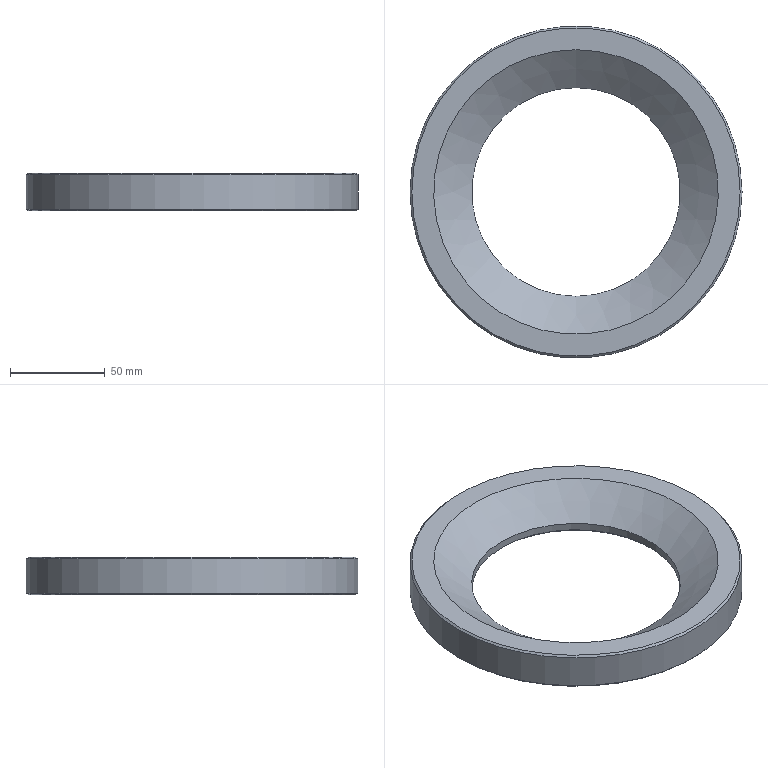Part | STEP file | solid 231 | 1 solid | 8 faces | box 175 x 175 x 20 mm | volume 232149 mm3 | cone 4 | cylinder 2 | plane 2 | commonest cylinder face diameters 110 x1 175 x1